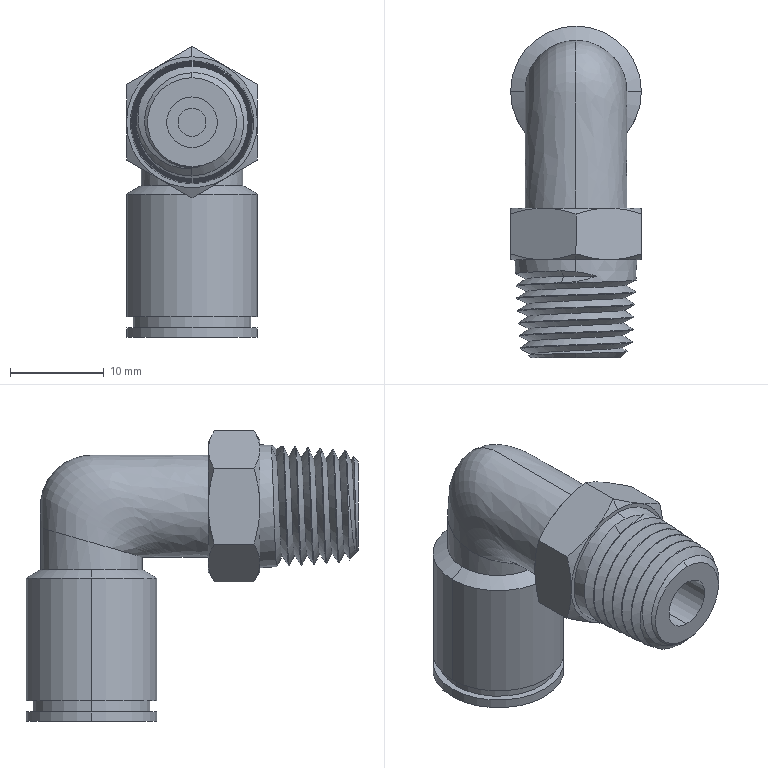Part | 1 solid | 70 faces | box 14 x 35.5 x 31.083 mm | volume 5084 mm3 | cone 32 | plane 18 | cylinder 14 | spline 6 | commonest cylinder face diameters 14 x4 3 x2 5.41 x2 8 x2 12.6 x2 12.8 x2